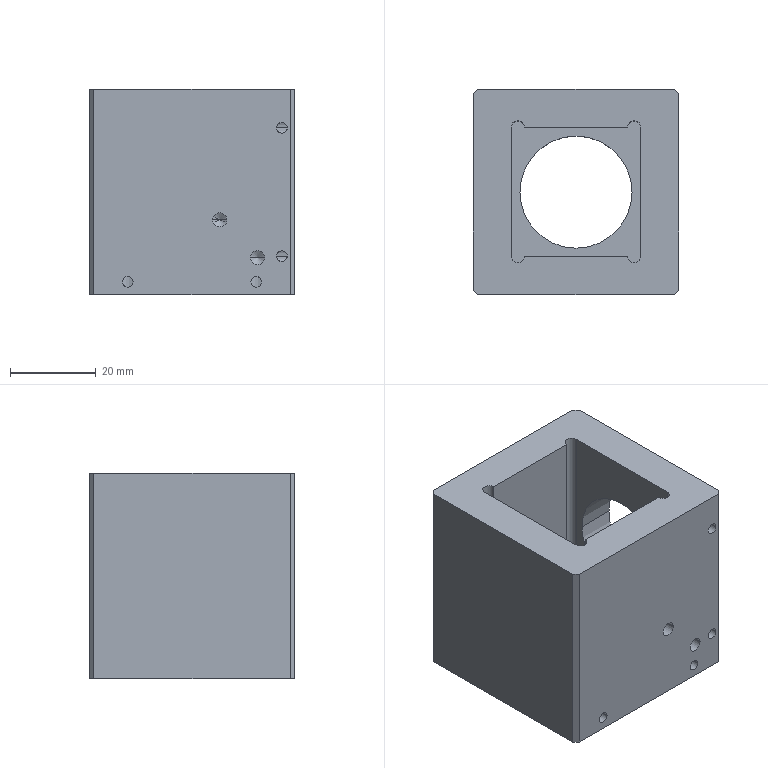NC program | NX | posted with a generic post | part box 48 x 48 x 48 mm
Lines 1 to 46 of 9644:
N10 G17 G21 G94 G90
(FLOOR_WALL_COPY , TOOL : D80)
N12 T19 M6
N14 G54
N16 G17 G0 G90 X-73. Y0. B0. C0. S6500 M3
N18 G43 Z30. H19
N20 Z3.
N22 G94 G1 Z0. F1500.
N24 X-68.
N26 X68.
N28 X73.
N30 Z3.
N32 G0 Z30.
N34 M5
(DRILLING_COPY_1 , TOOL : D6A45)
N36 T01 M6
N38 G54
N40 G17 G0 G90 X-13.6 Y15.1 B0. C0. S5000 M3
N42 G43 Z30. H1
N44 G94 G81 G98 Z-1. F350. R3.
N46 X13.6
N48 Y-15.1
N50 X-13.6
N52 G80
N54 G0 X-13.6 Y-15.1 Z30.
N56 M5
(DRILLING_COPY_1_COPY_1_1_COPY_1 , TOOL : 3.0ZT)
N58 T16 M6
N60 G54
N62 G17 G0 G90 X-13.6 Y15.1 B0. C0. S2000 M3
N64 G43 Z30. H16
N66 G94 G83 G98 Z-39.901 F100. Q2. R3.
N68 Y-15.1
N70 X13.6 Y15.1
N72 Y-15.1
N74 G80
N76 G0 X13.6 Y-15.1 Z30.
N78 M5